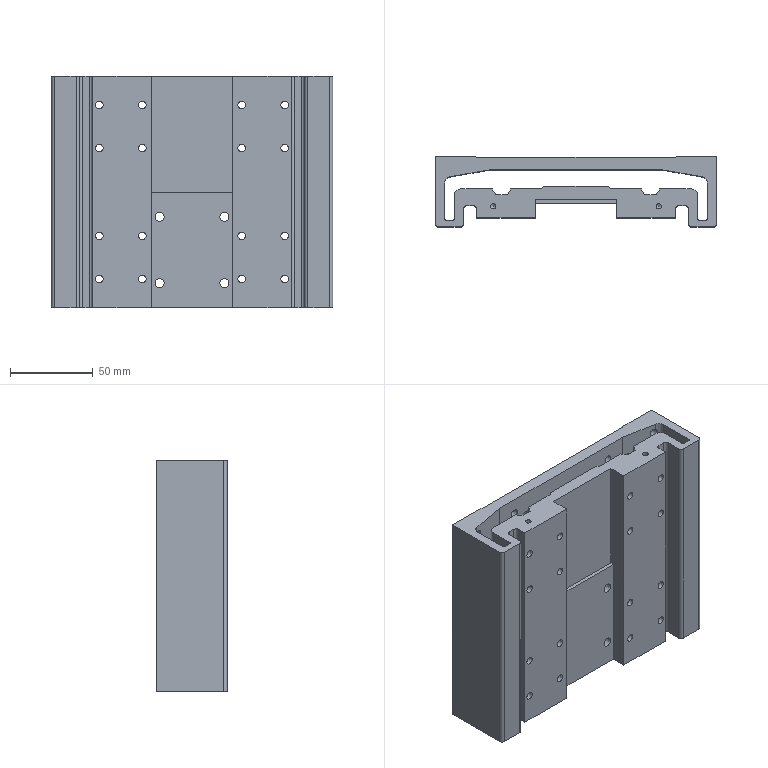Part | STEP file | 1 solid | 166 faces | box 170 x 42.5 x 140 mm | volume 521938 mm3 | cylinder 90 | plane 72 | cone 4 | commonest cylinder face diameters 8 x36 4.5 x16 4 x8 5 x8 9 x8 2 x4